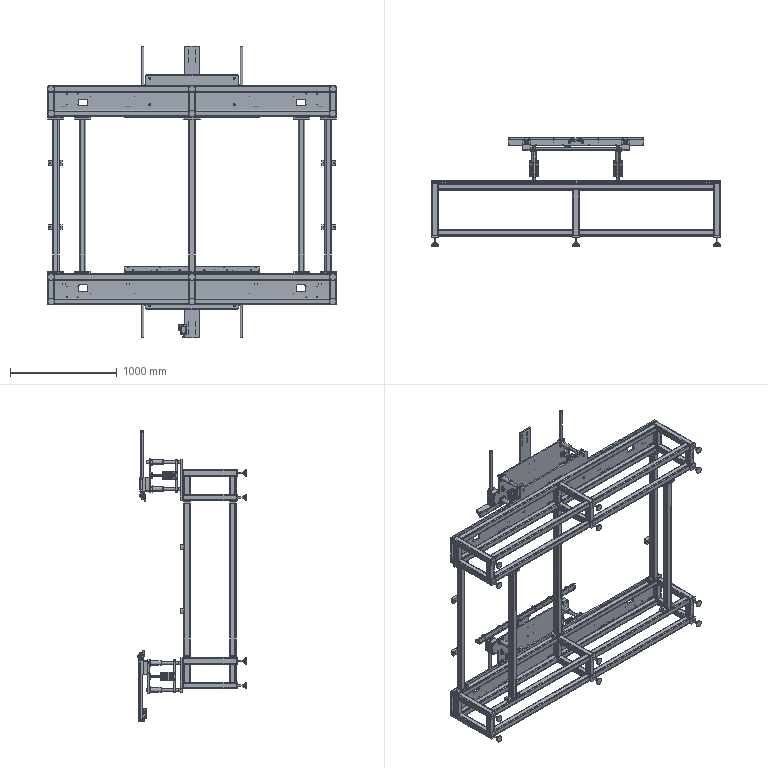Part | SolidWorks | features ReferencePattern 7, MirrorCompFeat 2, DerivedHolePattern 1 | 233 solids | 9276 faces | volume 88653077 mm3 | cylinder 4053 | plane 3459 | cone 1254 | spline 472 | torus 38 | commonest cylinder face diameters 6.8 x292 11 x264 10 x252 5 x250 6.6 x232 20 x192